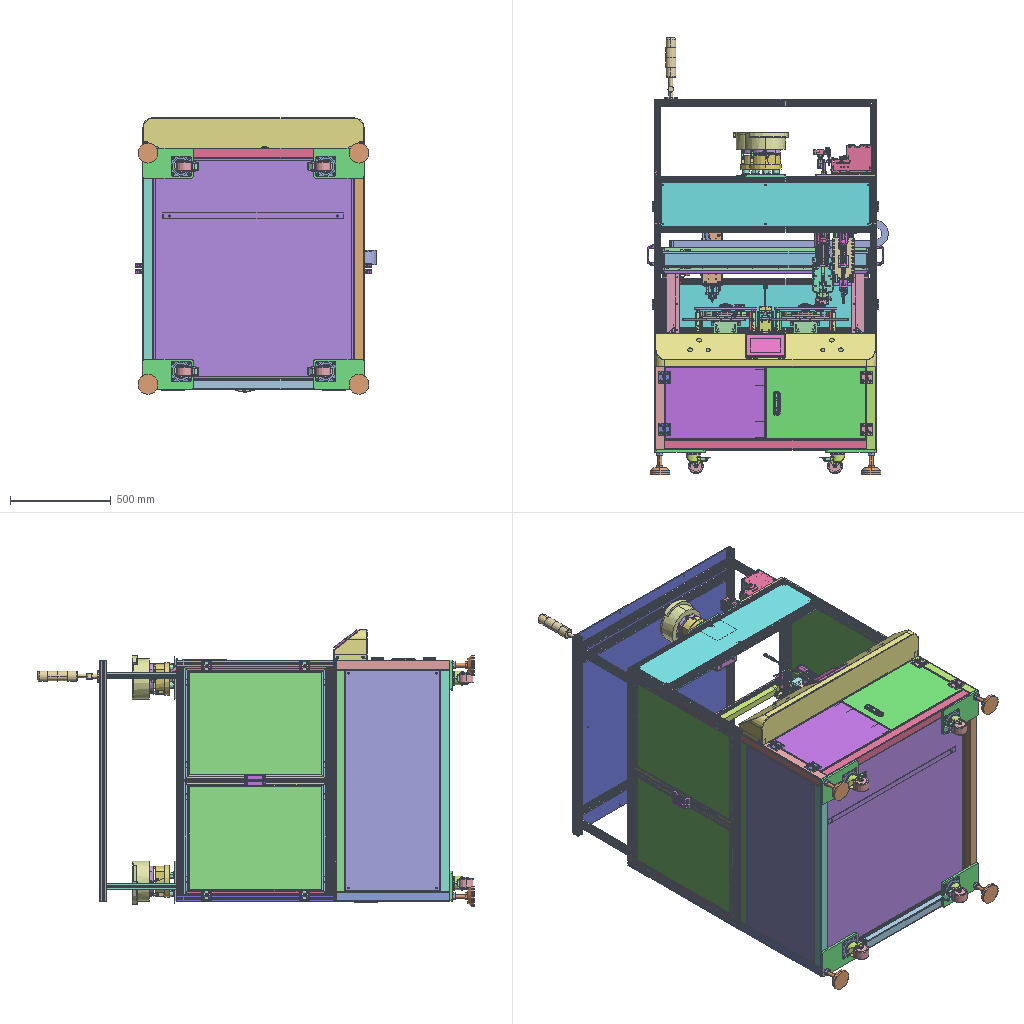Assembly | SolidWorks | 335 different items | 808 placed | box 1197 x 2172 x 1376 mm
Parts list (item | name | quantity | parent item | size | volume | features):
1 | 2MANIFOLD_SOLID_BREP_106 | x1 | - | - | - | -
2 | 2MANIFOLD_SOLID_BREP_107 | x1 | - | - | - | -
3 | 48-0003-001 Fuma Feeder | x1 | - | - | - | -
4 | (subassembly) | x2 | - | - | 2926027 mm3 | features InContextFeatHolder 1, LocalLPattern 1
5 | (subassembly) | x1 | in 48 | 106 x 347.75 x 115.5 mm | 813815 mm3 | -
6 | (subassembly) | x1 | in 48 | 118 x 296 x 169.5 mm | 901721 mm3 | features CompositeCurve 3
7 | (subassembly) | x1 | in 48 | - | 1242766 mm3 | features LocalLPattern 2, ReferencePattern 2, CompositeCurve 1
8 | (subassembly) | x1 | in 48 | - | 1493207 mm3 | features InContextFeatHolder 2, LocalLPattern 1, ReferencePattern 1
9 | (subassembly) | x2 | in 39 | 204.5 x 53 x 57 mm | 221430 mm3 | features CompositeCurve 1
10 | (subassembly) | x1 | in 5 | 163 x 64 x 71 mm | 272999 mm3 | features CompositeCurve 1
11 | (subassembly) | x1 | in 8 | 177 x 64 x 71 mm | 281305 mm3 | -
12 | (subassembly) | x4 | in 48 | 34 x 24 x 801 mm | 156547 mm3 | -
13 | (subassembly) | x1 | - | 160 x 158.001 x 310 mm | 1338981 mm3 | -
14 | (subassembly) | x1 | in 13 | - | - | -
15 | (subassembly) | x1 | in 5 | 75.5 x 39 x 43.25 mm | 30245 mm3 | -
16 | (subassembly) | x1 | in 13 | - | - | -
17 | (subassembly) | x1 | in 13 | - | - | -
18 | (subassembly) | x2 | in 39 | 72 x 24 x 16.5 mm | 14994 mm3 | features CompositeCurve 1
19 | (subassembly) | x2 | in 7 | 27 x 13 x 214 mm | 32172 mm3 | -
20 | (subassembly) | x2 | in 47, 52 | 128 x 25.22 x 23.366 mm | 18624 mm3 | features CompositeCurve 2
21 | (subassembly) | x1 | in 25 | 334 x 47.242 x 35.2 mm | 41085 mm3 | -
22 | (subassembly) | x2 | in 13 | 82 x 58 x 26 mm | 65223 mm3 | -
23 | (subassembly) | x2 | in 33 | 215 x 212 x 215 mm | 2165561 mm3 | -
24 | (subassembly) | x4 | in 28 | 109 x 58 x 20 mm | 97636 mm3 | -
25 | (subassembly) | x1 | in 48 | 108.9 x 604.66 x 99 mm | 644480 mm3 | -
26 | (subassembly) | x1 | in 49 | 532 x 358 x 55 mm | 405860 mm3 | -
27 | (subassembly) | x1 | in 49 | 549 x 358 x 41 mm | 436245 mm3 | -
28 | (subassembly) | x2 | in 4 | - | 4562071 mm3 | features InContextFeatHolder 23, LocalLPattern 2, ReferencePattern 2
29 | (subassembly) | x1 | in 49 | 1150 x 697 x 1255 mm | 10713372 mm3 | features ReferencePattern 18, MirrorCompFeat 5
30 | (subassembly) | x4 | in 38 | 51 x 717 x 593 mm | 2782623 mm3 | -
31 | (subassembly) | x1 | in 7 | 57.15 x 69.65 x 99 mm | 128417 mm3 | -
32 | (subassembly) | x5 | in 4, 6, 48 | 57.15 x 69.65 x 131 mm | 178571 mm3 | -
33 | (subassembly) | x2 | - | 215 x 224 x 215 mm | 2633576 mm3 | features ReferencePattern 12, MirrorCompFeat 2
34 | (subassembly) | x1 | in 25 | 28.124 x 80.028 x 32.009 mm | 13678 mm3 | features MirrorCompFeat 1, ReferencePattern 1
35 | (subassembly) | x1 | in 7 | 15 x 15 x 281 mm | 43646 mm3 | -
36 | (subassembly) | x2 | in 47, 52 | 27 x 13 x 80 mm | 13505 mm3 | -
37 | (subassembly) | x1 | in 5 | 24 x 50 x 40 mm | 9876 mm3 | -
38 | (subassembly) | x1 | - | - | 31701876 mm3 | features ReferencePattern 32, MirrorCompFeat 9, InContextFeatHolder 2, LocalLPattern 1
39 | (subassembly) | x2 | in 8, 48 | 174 x 106 x 364.833 mm | 559956 mm3 | features InContextFeatHolder 16
40 | (subassembly) | x2 | in 8 | 27 x 13 x 140 mm | 25516 mm3 | features LocalLPattern 1, ReferencePattern 1
41 | (subassembly) | x4 | in 28 | 50.06 x 40.7 x 50.06 mm | 29200 mm3 | -
42 | (subassembly) | x2 | in 28 | 63.5 x 60 x 65 mm | 47283 mm3 | features InContextFeatHolder 3
43 | (subassembly) | x2 | in 39 | - | - | -
44 | (subassembly) | x4 | in 28 | 50.005 x 46.2 x 50.005 mm | 37880 mm3 | features InContextFeatHolder 3
45 | (subassembly) | x2 | in 13 | - | - | -
46 | (subassembly) | x2 | in 13 | - | - | -
47 | (subassembly) | x1 | - | 247.423 x 78.5 x 242 mm | 390911 mm3 | features InContextFeatHolder 6, CompositeCurve 2
48 | (subassembly) | x1 | - | - | - | features InContextFeatHolder 20, ReferencePattern 6, LocalLPattern 2, AEMSimFeature 1, MirrorCompFeat 1
49 | (subassembly) | x1 | - | - | 25832975 mm3 | features InContextFeatHolder 16, ReferencePattern 13, MirrorCompFeat 5
50 | (subassembly) | x1 | - | - | - | -
51 | (subassembly) | x5 | in 4, 6, 48 | 86 x 30 x 36 mm | 32834 mm3 | -
52 | (subassembly) | x1 | - | 247.56 x 78.5 x 242 mm | 391168 mm3 | features CompositeCurve 2
53 | (subassembly) | x4 | in 13 | - | - | -
54 | (subassembly) | x8 | in 30 | 50 x 50 x 12 mm | 15792 mm3 | -
55 | - | x1 | in 6 | 15 x 15 x 180 mm | 39722 mm3 | features ICE 2, Extrusion 1, LPattern 1
56 | - | x2 | in 48 | 83 x 297.5 x 153 mm | 132510 mm3 | features ICE 3, Fillet 2, Shell 2, Chamfer 1, Extrusion 1, HoleWzd 1
57 | - | x4 | in 4 | 122 x 65.5 x 4 mm | 31619 mm3 | features Extrusion 1, Fillet 1
58 | - | x4 | in 4, 48 | 14 x 33 x 12 mm | 507.507 mm3 | features MoveFace 7, ICE 2, BaseBody 1, Fillet 1
59 | - | x4 | in 4, 48 | 19 x 20 x 50 mm | 3170 mm3 | features Fillet 3, ICE 2, ExtruThin 1
60 | - | x4 | in 38 | 3 x 60 x 50 mm | 5947 mm3 | features HoleWzd 2, Fillet 1, FlatPattern 1, ICE 1, SMBaseFlange 1, SheetMetal 1
61 | - | x1 | in 6 | 30 x 50 x 100 mm | 12860 mm3 | features HoleWzd 2, EdgeFlange 1, Fillet 1, FlatPattern 1, SMBaseFlange 1, SheetMetal 1
62 | - | x2 | in 47, 52 | 5 x 12 x 25 mm | 1176 mm3 | features Fillet 4, ICE 4, Cut 1, Extrusion 1, HoleWzd 1
63 | - | x4 | in 47, 52 | 3 x 67 x 43.5 mm | 6128 mm3 | features ICE 5, Fillet 4, Extrusion 1, HoleWzd 1, LPattern 1
64 | - | x2 | in 47, 52 | 3 x 42 x 25 mm | 2502 mm3 | features Fillet 3, ICE 3, Cut 1, Extrusion 1, HoleWzd 1
65 | - | x2 | in 47, 52 | 1 x 48 x 65 mm | 2915 mm3 | features ICE 8, Fillet 2, Chamfer 1, Extrusion 1, HoleWzd 1
66 | - | x1 | in 25 | 34 x 19.5 x 56.8 mm | 30598 mm3 | features ICE 2, Extrusion 1
67 | - | x2 | in 33 | 184 x 160 x 140 mm | 320249 mm3 | features Fillet 2, Extrusion 1, ICE 1
68 | - | x4 | in 39 | 3 x 36 x 65 mm | 4945 mm3 | features Fillet 2, HoleWzd 2, ICE 2, Extrusion 1
69 | - | x2 | in 39 | 33 x 59 x 3 mm | 3614 mm3 | features Cut 4, ICE 4, Fillet 3, MoveFace 2, Extrusion 1, HoleWzd 1
70 | - | x2 | in 39 | 35 x 23 x 3 mm | 2147 mm3 | features Fillet 2, MoveFace 2, Extrusion 1, ICE 1
71 | - | x2 | in 39 | 14.5 x 3 x 15 mm | 477.667 mm3 | features Extrusion 1, Fillet 1, ICE 1
72 | - | x2 | in 39 | 43 x 37 x 0.8 mm | 1152 mm3 | features ICE 5, HoleWzd 2, Cut 1, Extrusion 1, Fillet 1, MirrorPattern 1, MoveFace 1
73 | - | x1 | in 7 | 30 x 50 x 66 mm | 9795 mm3 | features HoleWzd 2, EdgeFlange 1, Fillet 1, FlatPattern 1, SMBaseFlange 1, SheetMetal 1
74 | - | x1 | in 7 | 33.8 x 20 x 11 mm | 767.773 mm3 | features EdgeFlange 2, ICE 2, Fillet 1, FlatPattern 1, SMBaseFlange 1, SheetMetal 1
75 | - | x1 | in 25 | 25 x 53 x 20 mm | 8091 mm3 | features ICE 7, HoleWzd 4, 3DProfileFeature 2, Chamfer 2, Extrusion 1, Fillet 1, RevCut 1, Revolution 1
76 | - | x2 | in 5 | 12 x 120 x 12 mm | 13432 mm3 | features Chamfer 1, Extrusion 1, HoleWzd 1, ICE 1
77 | - | x2 | in 39 | 5.7 x 10.3 x 5.7 mm | 17.455 mm3 | features Helix 1, ICE 1, Sweep 1
78 | - | x1 | in 5 | 24 x 65 x 25 mm | 25326 mm3 | features HoleWzd 3, ICE 2, Chamfer 1, Extrusion 1, MirrorPattern 1
79 | - | x1 | in 37 | 11 x 32 x 11 mm | 1736 mm3 | features Chamfer 5, ICE 4, HoleWzd 3, RevCut 2, Extrusion 1
80 | - | x2 | in 39 | 10 x 60 x 10 mm | 1412 mm3 | features Chamfer 1, Extrusion 1, Fillet 1, ICE 1
81 | - | x2 | in 39 | 3 x 145 x 3 mm | 797.28 mm3 | features ICE 4, Chamfer 2, MoveFace 2, Extrusion 1
82 | - | x2 | in 39 | 15 x 13 x 30 mm | 3613 mm3 | features ICE 4, Chamfer 1, Extrusion 1, HoleWzd 1
83 | - | x2 | in 48 | 150 x 300 x 20 mm | 887361 mm3 | features HoleWzd 5, MirrorPattern 2, Chamfer 1, Extrusion 1
84 | - | x1 | in 48 | 15 x 150 x 1018 mm | 2102309 mm3 | features HoleWzd 6, ICE 3, MirrorPattern 2, Chamfer 1, Extrusion 1, Fillet 1
85 | - | x1 | in 48 | 1000 x 118 x 12 mm | 1222730 mm3 | features HoleWzd 11, ICE 3, MirrorPattern 3, Chamfer 2, Cut 2, Fillet 2, LPattern 2, MoveFace 2, Extrusion 1
86 | - | x4 | in 48 | 75 x 4 x 8 mm | 2157 mm3 | features Chamfer 5, ICE 4, HoleWzd 2, Extrusion 1, Fillet 1
87 | - | x1 | in 48 | 150 x 133 x 15 mm | 253404 mm3 | features HoleWzd 4, ICE 3, Extrusion 1, Fillet 1, MirrorPattern 1
88 | - | x2 | in 39 | 13.6 x 2 x 2 mm | 42.623 mm3 | features Extrusion 1, Fillet 1
89 | - | x2 | in 48 | 65 x 35 x 85 mm | 63871 mm3 | features HoleWzd 5, ICE 3, Extrusion 1
90 | - | x2 | in 48 | 70 x 112 x 15 mm | 96794 mm3 | features HoleWzd 8, ICE 4, MirrorPattern 2, Extrusion 1
91 | - | x4 | in 48 | 12 x 70 x 45 mm | 30841 mm3 | features HoleWzd 5, Extrusion 1, MirrorPattern 1
92 | - | x2 | in 48 | 50 x 95 x 20 mm | 89595 mm3 | features HoleWzd 2, Chamfer 1, Extrusion 1
93 | - | x1 | in 48 | 150 x 133 x 15 mm | 252829 mm3 | features HoleWzd 4, ICE 3, Extrusion 1, Fillet 1, MirrorPattern 1
94 | - | x4 | in 4, 48 | 50 x 16 x 5.5 mm | 4295 mm3 | features Chamfer 1, Extrusion 1, HoleWzd 1
95 | - | x2 | in 4 | 150 x 200 x 10 mm | 295428 mm3 | features HoleWzd 3, ICE 3, Extrusion 1, Fillet 1, LPattern 1
96 | - | x1 | in 5 | 106 x 235 x 10 mm | 238418 mm3 | features HoleWzd 7, ICE 5, Fillet 2, Extrusion 1, LPattern 1, MirrorPattern 1, MoveFace 1
97 | - | x1 | in 5 | 82 x 10 x 82 mm | 53941 mm3 | features HoleWzd 7, Extrusion 1, Fillet 1, ICE 1, MirrorPattern 1
98 | - | x1 | in 5 | 26 x 35 x 15.8 mm | 2299 mm3 | features ICE 10, Fillet 6, Chamfer 1, Extrusion 1, HoleWzd 1, MoveFace 1
99 | - | x2 | in 48 | 30 x 24 x 30 mm | 11200 mm3 | features ICE 11, Chamfer 4, CirPattern 1, HoleWzd 1, Revolution 1
100 | - | x1 | in 5 | 26 x 35 x 15.8 mm | 2299 mm3 | features MirrorStock 1
101 | - | x1 | in 5 | 65 x 10 x 32 mm | 16925 mm3 | features HoleWzd 3, ICE 3, Extrusion 1, Fillet 1
102 | - | x1 | in 5 | 95 x 12 x 100 mm | 64491 mm3 | features HoleWzd 6, ICE 3, Fillet 2, Extrusion 1
103 | - | x1 | in 8 | 72 x 10 x 64 mm | 33293 mm3 | features HoleWzd 5, ICE 5, Fillet 2, Extrusion 1
104 | - | x1 | in 37 | 24 x 24 x 40 mm | 8141 mm3 | features ICE 7, Chamfer 4, HoleWzd 4, Extrusion 1, RevCut 1
105 | - | x1 | in 8 | 95 x 170.5 x 10 mm | 143560 mm3 | features HoleWzd 8, ICE 8, Fillet 4, MoveFace 2, Cut 1, Extrusion 1, MirrorPattern 1
106 | - | x1 | in 8 | 180 x 190 x 10 mm | 333166 mm3 | features HoleWzd 6, ICE 2, Extrusion 1, Fillet 1, LPattern 1
107 | - | x3 | in 4, 6 | 86 x 58 x 5 mm | 19221 mm3 | features ICE 5, HoleWzd 4, 3DProfileFeature 2, MirrorPattern 2, Chamfer 1, Cut 1, Extrusion 1, LPattern 1
108 | - | x1 | in 6 | 238.67 x 16.67 x 12 mm | 3738 mm3 | features Extrusion 1
109 | - | x1 | in 6 | 86 x 24 x 36 mm | 22794 mm3 | features ICE 7, Chamfer 1, Extrusion 1, RevCut 1
110 | - | x2 | in 6 | 100 x 65 x 8 mm | 46552 mm3 | features Chamfer 4, MoveFace 3, Fillet 2, HoleWzd 2, ICE 2, Extrusion 1
111 | - | x2 | in 47, 52 | 12 x 55 x 140 mm | 81002 mm3 | features ICE 2, Chamfer 1, Extrusion 1, HoleWzd 1, MirrorPattern 1
112 | - | x4 | in 47, 52 | 55 x 60 x 10 mm | 32595 mm3 | features Extrusion 1, HoleWzd 1, MirrorPattern 1
113 | - | x2 | in 47, 52 | 12 x 55 x 152 mm | 91517 mm3 | features HoleWzd 6, ICE 5, MirrorPattern 2, Chamfer 1, Cut 1, Extrusion 1
114 | - | x6 | in 39, 47, 52 | 20 x 10 x 8 mm | 1332 mm3 | features HoleWzd 2, Extrusion 1, ICE 1, MoveFace 1
115 | - | x2 | in 47, 52 | 10 x 55 x 35 mm | 16084 mm3 | features HoleWzd 3, Chamfer 1, Extrusion 1, ICE 1, MirrorPattern 1
116 | - | x2 | in 47, 52 | 10 x 48 x 20 mm | 8641 mm3 | features Extrusion 1, HoleWzd 1
117 | - | x3 | in 39, 47 | 25 x 55 x 12 mm | 15520 mm3 | features ICE 4, Chamfer 2, Fillet 2, HoleWzd 2, MirrorPattern 2, Extrusion 1
118 | - | x1 | in 47 | 20 x 48 x 65 mm | 52206 mm3 | features ICE 6, HoleWzd 3, Chamfer 2, Fillet 2, Extrusion 1, MoveFace 1
119 | - | x1 | in 52 | 20 x 48 x 65 mm | 52425 mm3 | features ICE 6, HoleWzd 3, Chamfer 2, Fillet 2, Extrusion 1, MoveFace 1
120 | - | x3 | in 39, 52 | 25 x 55 x 12 mm | 15456 mm3 | features ICE 4, Chamfer 2, Fillet 2, HoleWzd 2, MirrorPattern 2, Extrusion 1
121 | - | x1 | in 8 | 96 x 120 x 10 mm | 109019 mm3 | features HoleWzd 2, Extrusion 1, Fillet 1, ICE 1
122 | - | x2 | in 39 | 7 x 7 x 42.5 mm | 1702 mm3 | features Chamfer 3, ICE 3, Extrusion 1, MoveFace 1
123 | - | x2 | in 39 | 52 x 37 x 19 mm | 25597 mm3 | features HoleWzd 8, ICE 8, MoveFace 8, Chamfer 2, Extrusion 1, Fillet 1, MirrorPattern 1, RefAxis 1
124 | - | x2 | in 39 | 7 x 8.44 x 8 mm | 333.679 mm3 | features ICE 5, Chamfer 2, Extrusion 1, MoveFace 1
125 | - | x2 | in 39 | 5 x 8.4 x 7.9 mm | 224.151 mm3 | features ICE 5, Chamfer 2, MoveFace 2, Extrusion 1
126 | - | x2 | in 39 | 22 x 12.5 x 10 mm | 1861 mm3 | features HoleWzd 2, ICE 2, Chamfer 1, Extrusion 1, MoveFace 1
127 | - | x2 | in 39 | 43 x 37 x 12 mm | 14568 mm3 | features HoleWzd 6, ICE 4, MoveFace 2, Chamfer 1, Extrusion 1, LPattern 1, RefAxis 1
128 | - | x2 | in 39 | 33 x 15 x 45 mm | 11629 mm3 | features Chamfer 1, Extrusion 1, HoleWzd 1, ICE 1
129 | - | x2 | in 39 | 95 x 12 x 63 mm | 36710 mm3 | features HoleWzd 7, ICE 3, Fillet 2, Extrusion 1
130 | - | x2 | in 39 | 106 x 235 x 10 mm | 201663 mm3 | features ICE 18, HoleWzd 12, Fillet 5, MoveFace 3, LPattern 2, MirrorPattern 2, Extrusion 1
131 | - | x2 | in 39 | 96 x 211.5 x 10 mm | 163638 mm3 | features ICE 21, HoleWzd 16, Fillet 5, MoveFace 3, LPattern 2, MirrorPattern 2, Chamfer 1, Extrusion 1
132 | - | x1 | in 7 | 100 x 75 x 8 mm | 49957 mm3 | features Cut 2, HoleWzd 2, Chamfer 1, Extrusion 1, Fillet 1, ICE 1
133 | - | x1 | in 7 | 100 x 71.5 x 8 mm | 49163 mm3 | features Chamfer 1, Cut 1, Extrusion 1, Fillet 1, HoleWzd 1, ICE 1
134 | - | x1 | in 7 | 86 x 61.5 x 12 mm | 38021 mm3 | features HoleWzd 5, ICE 5, Chamfer 4, MoveFace 3, Extrusion 1
135 | - | x1 | in 7 | 86 x 61.5 x 15 mm | 44493 mm3 | features ICE 7, HoleWzd 4, Chamfer 3, MoveFace 2, Extrusion 1
136 | - | x1 | in 7 | 106 x 56 x 80 mm | 252675 mm3 | features ICE 9, HoleWzd 7, Chamfer 4, CirPattern 2, Cut 2, Extrusion 1, LPattern 1
137 | - | x3 | in 38 | 215 x 1038 x 6 mm | 1337506 mm3 | features Extrusion 1, Fillet 1, HoleWzd 1
138 | - | x1 | in 38 | 1100 x 6 x 1200 mm | 7913109 mm3 | features HoleWzd 2, ICE 2, Extrusion 1, Fillet 1
139 | - | x4 | in 30 | 6 x 677 x 528 mm | 2144688 mm3 | features Chamfer 1, Extrusion 1
140 | - | x2 | in 33 | 200 x 12 x 200 mm | 468015 mm3 | features Cut 1, Extrusion 1, Fillet 1
141 | - | x1 | in 6 | 45 x 8 x 15 mm | 5130 mm3 | features Extrusion 1, HoleWzd 1, ICE 1
142 | - | x2 | in 7 | 12 x 12 x 15 mm | 1371 mm3 | features Extrusion 1, HoleWzd 1
143 | - | x2 | in 48 | 79 x 6 x 1020 mm | 209920 mm3 | features Cut 1, Extrusion 1, MirrorPattern 1
144 | - | x2 | in 4 | 143.4 x 35.1 x 60 mm | 99066 mm3 | features HoleWzd 8, MirrorPattern 5, ICE 3, Chamfer 1, Extrusion 1, LPattern 1
145 | - | x2 | in 4 | 120 x 12 x 1000 mm | 423626 mm3 | features Extrusion 1, HoleWzd 1, ICE 1, MirrorPattern 1
146 | - | x1 | in 38 | 1100 x 780 x 1200 mm | 5922757 mm3 | features ICE 14, 3DProfileFeature 2, HoleWzd 2, WeldMemberFeat 2, WeldmentFeature 1
147 | - | x4 | in 30 | 30 x 15 x 717 mm | 163021 mm3 | features Extrusion 1, HoleWzd 1, ICE 1
148 | - | x4 | in 30 | 30 x 15 x 717 mm | 163444 mm3 | features Extrusion 1, HoleWzd 1, ICE 1
149 | - | x4 | in 29 | 100 x 106 x 139 mm | 279325 mm3 | features BaseBody 5
150 | - | x8 | in 30 | 30 x 15 x 568 mm | 128082 mm3 | features Extrusion 1, HoleWzd 1, ICE 1
151 | - | x4 | in 38 | 1040 x 30 x 30 mm | 414964 mm3 | features WeldMemberFeat 1, WeldmentFeature 1
152 | - | x1 | in 6 | 100 x 46 x 280 mm | 353239 mm3 | features HoleWzd 7, ICE 5, MirrorPattern 5, 3DProfileFeature 3, Fillet 3, LPattern 3, Cut 2, Chamfer 1, Extrusion 1
153 | - | x1 | in 6 | 106 x 38 x 60 mm | 90816 mm3 | features HoleWzd 7, 3DProfileFeature 4, ICE 4, Chamfer 1, Extrusion 1, LPattern 1, MirrorPattern 1, MoveFace 1
154 | - | x1 | in 6 | 79 x 6 x 296 mm | 60805 mm3 | features Cut 1, Extrusion 1, MirrorPattern 1
155 | - | x1 | in 7 | 100 x 46 x 306 mm | 422449 mm3 | features HoleWzd 8, ICE 3, 3DProfileFeature 1, Extrusion 1, LPattern 1, MirrorPattern 1
156 | - | x1 | in 7 | 79 x 6 x 306 mm | 62238 mm3 | features ICE 4, Extrusion 1, HoleWzd 1
157 | - | x1 | in 7 | 6 x 9 x 200 mm | 5872 mm3 | features ICE 3, Extrusion 1
158 | - | x5 | in 51 | 86 x 24 x 36 mm | 22794 mm3 | features ICE 7, Chamfer 1, Extrusion 1, RevCut 1
159 | - | x2 | in 4 | 30 x 24 x 30 mm | 11209 mm3 | features ICE 12, Chamfer 4, CirPattern 1, HoleWzd 1, Revolution 1
160 | - | x1 | in 48 | 781.5 x 119 x 54 mm | 397201 mm3 | features ICE 12, Fillet 2, HoleWzd 2, Shell 1, Sweep 1
161 | - | x5 | in 51 | 30 x 21 x 30 mm | 8531 mm3 | features Chamfer 2, ICE 2, MirrorPattern 1, Revolution 1
162 | - | x4 | in 4 | 45 x 8 x 15 mm | 5130 mm3 | features Extrusion 1, HoleWzd 1, ICE 1
163 | - | x2 | in 4 | 100 x 46 x 1000 mm | 1360190 mm3 | features HoleWzd 6, ICE 6, MirrorPattern 4, Fillet 3, LPattern 3, Chamfer 1, Extrusion 1
164 | - | x2 | in 28 | 15 x 215 x 215 mm | 479091 mm3 | features ICE 5, HoleWzd 3, Cut 2, Fillet 2, LPattern 2, Chamfer 1, Extrusion 1, RefAxis 1, RevCut 1
165 | - | x2 | in 28 | 10.7 x 214.9 x 214.8 mm | 326451 mm3 | features MoveCopyBody 6, ICE 5, Fillet 2, LPattern 2, MoveFace 2, Chamfer 1, Cut 1, Extrusion 1, Stock 1
166 | - | x2 | in 28 | 10.7 x 214.9 x 214.8 mm | 309606 mm3 | features ICE 6, MoveCopyBody 6, Cut 3, Fillet 3, Chamfer 1, Extrusion 1, LPattern 1, MoveFace 1, Stock 1
167 | - | x2 | in 28 | 13.1 x 214.9 x 214.8 mm | 329886 mm3 | features ICE 7, MoveCopyBody 6, Fillet 3, Cut 2, Chamfer 1, Extrusion 1, LPattern 1, MoveFace 1, Stock 1
168 | - | x2 | in 28 | 10 x 225 x 237 mm | 510039 mm3 | features HoleWzd 6, Chamfer 2, MirrorPattern 2, MoveFace 2, Extrusion 1, ICE 1
169 | - | x2 | in 28 | 25 x 225 x 10 mm | 52898 mm3 | features Chamfer 2, HoleWzd 2, Extrusion 1, Fillet 1
170 | - | x2 | in 28 | 25 x 10 x 210 mm | 50226 mm3 | features Extrusion 1, HoleWzd 1, ICE 1
171 | - | x2 | in 28 | 8 x 215 x 311 mm | 385506 mm3 | features Cut 2, Fillet 2, ICE 2, MirrorPattern 2, MoveFace 2, Chamfer 1, Extrusion 1, LPattern 1
172 | - | x4 | in 28 | 98 x 10 x 157.5 mm | 116638 mm3 | features HoleWzd 4, Chamfer 1, Extrusion 1, Fillet 1, ICE 1
173 | - | x2 | in 28 | 25 x 225 x 10 mm | 52898 mm3 | features MirrorStock 1
174 | - | x3 | in 28 | 10 x 35 x 120 mm | 41153 mm3 | features Chamfer 1, Extrusion 1, HoleWzd 1, ICE 1, LPattern 1
175 | - | x2 | in 28 | 25 x 215 x 215 mm | 792326 mm3 | features ICE 12, MoveCopyBody 7, LPattern 6, MoveFace 5, Chamfer 4, Cut 2, Fillet 2, Stock 2, Extrusion 1, HoleWzd 1
176 | - | x2 | in 28 | 98 x 10 x 157.5 mm | 116638 mm3 | features MirrorStock 1
177 | - | x2 | in 28 | 25 x 215 x 215 mm | 773722 mm3 | features ICE 14, MoveCopyBody 7, LPattern 5, MoveFace 5, Chamfer 3, Cut 2, Stock 2, Extrusion 1, HoleWzd 1
178 | - | x2 | in 28 | 25 x 215 x 215 mm | 796831 mm3 | features ICE 14, MoveCopyBody 7, MoveFace 6, Chamfer 4, LPattern 4, Cut 3, Fillet 3, Stock 2, Extrusion 1, HoleWzd 1
179 | - | x1 | in 6 | 19 x 17 x 50 mm | 3062 mm3 | features Fillet 3, ICE 2, ExtruThin 1
180 | - | x1 | in 6 | 50 x 16 x 3 mm | 2365 mm3 | features Chamfer 1, Extrusion 1, HoleWzd 1
181 | - | x4 | in 44 | 16.9 x 32 x 32 mm | 11867 mm3 | features ICE 6, Cut 1, Extrusion 1, Fillet 1
182 | - | x1 | in 6 | 14 x 25 x 12 mm | 411.507 mm3 | features MoveFace 3, ICE 2, BaseBody 1, Fillet 1
183 | - | x1 | in 6 | 30 x 24 x 30 mm | 11209 mm3 | features ICE 12, Chamfer 4, CirPattern 1, HoleWzd 1, Revolution 1
184 | - | x2 | in 25 | 20 x 16 x 16 mm | 3358 mm3 | features Extrusion 1
185 | - | x1 | in 25 | 40 x 17 x 58.5 mm | 18418 mm3 | features ICE 9, Chamfer 6, HoleWzd 5, MirrorPattern 3, Fillet 2, MoveFace 2, Extrusion 1
186 | - | x2 | in 48 | 880.84 x 28.34 x 15 mm | 31689 mm3 | features Extrusion 1
187 | - | x1 | in 35 | 15 x 15 x 281 mm | 43646 mm3 | features RevCut 4, Chamfer 2, Extrusion 1, ICE 1
188 | - | x1 | - | 18 x 55 x 99.9 mm | 49289 mm3 | features BaseBody 1
189 | - | x2 | in 6, 7 | 8.882 x 97 x 8 mm | 1277 mm3 | features BaseBody 3, ICE 1, RefAxis 1
190 | - | x1 | in 10 | 8 x 31.177 x 27 mm | 3647 mm3 | features BaseBody 1
191 | - | x1 | in 11 | 8 x 31.177 x 27 mm | 3647 mm3 | features BaseBody 1
192 | - | x6 | in 41, 42 | 14.5 x 33 x 33 mm | 10024 mm3 | features Cut 2, ICE 2, CirPattern 1, Extrusion 1
193 | - | x1 | in 10 | 11 x 31.177 x 27 mm | 4519 mm3 | features BaseBody 1
194 | - | x1 | in 10 | 31 x 36 x 36 mm | 21772 mm3 | features BaseBody 1
195 | - | x1 | in 11 | 41 x 36 x 36 mm | 28650 mm3 | features BaseBody 1
196 | - | x1 | in 11 | 177 x 50 x 50 mm | 73758 mm3 | features BaseBody 1
197 | - | x1 | in 11 | 80.5 x 71 x 64 mm | 175247 mm3 | features BaseBody 1
198 | - | x1 | in 10 | 163 x 50 x 50 mm | 86233 mm3 | features BaseBody 1
199 | - | x1 | in 10 | 70.5 x 71 x 64 mm | 156826 mm3 | features BaseBody 1
200 | - | x2 | in 20 | 107 x 18 x 18 mm | 12758 mm3 | features BaseBody 1
201 | - | x2 | in 20 | 110.9 x 11.5 x 11.5 mm | 4064 mm3 | features BaseBody 1
202 | - | x1 | in 13 | - | - | features RefSurface 77
203 | - | x2 | in 20 | 6 x 25.403 x 22 mm | 1471 mm3 | features BaseBody 1
204 | - | x2 | in 20 | 5 x 11.547 x 10 mm | 331.011 mm3 | features BaseBody 1
205 | - | x1 | in 21 | 6 x 25.403 x 22 mm | 1471 mm3 | features BaseBody 1
206 | - | x1 | in 21 | 5 x 11.547 x 10 mm | 331.011 mm3 | features BaseBody 1
207 | - | x1 | in 21 | 334 x 15.5 x 15.5 mm | 11530 mm3 | features BaseBody 1
208 | - | x1 | in 21 | 167 x 20 x 20 mm | 22187 mm3 | features BaseBody 1
209 | - | x1 | in 21 | 5 x 11.547 x 10 mm | 331.011 mm3 | features BaseBody 1
210 | - | x1 | in 21 | 66 x 15 x 15 mm | 8114 mm3 | features BaseBody 1
211 | - | x2 | in 22 | 49 x 26 x 58 mm | 50658 mm3 | features BaseBody 1
212 | - | x2 | in 22 | 59.5 x 22 x 56 mm | 14565 mm3 | features BaseBody 1
213 | - | x1 | in 38 | 900 x 35 x 34 mm | 955428 mm3 | features Extrusion 1, HoleWzd 1, ICE 1, MirrorPattern 1
214 | - | x4 | in 24 | 99 x 20 x 58 mm | 74621 mm3 | features BaseBody 1
215 | - | x4 | in 24 | 103.6 x 18 x 56 mm | 23014 mm3 | features BaseBody 1
216 | - | x2 | in 39 | 6 x 6 x 55 mm | 1555 mm3 | features Extrusion 1
217 | - | x4 | in 44 | 32 x 33.3 x 32 mm | 14832 mm3 | features ICE 2, BaseBody 1, MoveFace 1
218 | - | x6 | in 41, 42 | 33 x 35.1 x 33 mm | 19096 mm3 | features MoveFace 3, BaseBody 1, CirPattern 1, HoleWzd 1
219 | - | x1 | in 8 | 17 x 19.6 x 45 mm | 6216 mm3 | features BaseBody 1, MoveFace 1
220 | - | x2 | in 47, 52 | 15.5 x 15.5 x 18 mm | 2342 mm3 | features BaseBody 1
221 | - | x1 | in 13 | 98 x 66 x 12 mm | 42190 mm3 | features ICE 6, HoleWzd 4, Chamfer 2, Extrusion 1, MirrorPattern 1
222 | - | x4 | in 41 | 1.99 x 13.6 x 1.99 mm | 41.809 mm3 | features BaseBody 1
223 | - | x2 | in 28 | 12 x 31.537 x 120 mm | 3389 mm3 | features Fillet 4, Extrusion 1, ICE 1
224 | - | x4 | in 13 | 13 x 6 x 13 mm | 944.273 mm3 | features Chamfer 1, Extrusion 1, HoleWzd 1
225 | - | x1 | in 13 | 30 x 12 x 62 mm | 15056 mm3 | features ICE 3, HoleWzd 2, Chamfer 1, Extrusion 1, MirrorPattern 1
226 | - | x1 | in 13 | 126 x 12 x 25 mm | 32289 mm3 | features ICE 4, Chamfer 1, Extrusion 1, HoleWzd 1, MirrorPattern 1
227 | - | x1 | in 5 | 53 x 53 x 22 mm | 15531 mm3 | features ICE 3, Chamfer 1, Extrusion 1
228 | - | x1 | in 5 | 15 x 15 x 47 mm | 1444 mm3 | features 3DProfileFeature 1, Helix 1, RefAxis 1, Sweep 1
229 | - | x8 | in 48 | 53 x 53 x 52 mm | 37709 mm3 | features ICE 3, Chamfer 1, Extrusion 1
230 | - | x1 | in 38 | 60 x 307 x 60 mm | 453785 mm3 | features BaseBody 1
231 | - | x1 | in 13 | 160 x 12 x 300 mm | 482018 mm3 | features HoleWzd 12, ICE 6, Chamfer 1, Extrusion 1, Fillet 1, MirrorPattern 1
232 | - | x1 | in 13 | 14 x 25 x 15 mm | 2174 mm3 | features ICE 6, Chamfer 2, RevCut 2, Extrusion 1, MirrorPattern 1
233 | - | x4 | in 41 | 1.99 x 13.6 x 1.99 mm | 41.809 mm3 | features BaseBody 1
234 | - | x1 | in 13 | 14 x 29 x 15 mm | 2672 mm3 | features Chamfer 4, ICE 4, Extrusion 1, HoleWzd 1
235 | - | x1 | in 13 | 42 x 10 x 29 mm | 6453 mm3 | features HoleWzd 3, ICE 3, Fillet 2, Chamfer 1, Extrusion 1
236 | - | x1 | in 13 | 56 x 25 x 26 mm | 11259 mm3 | features ICE 5, Fillet 2, HoleWzd 2, Chamfer 1, Extrusion 1
237 | - | x1 | in 49 | 200 x 145 x 43 mm | 1064774 mm3 | features ICE 5, Fillet 3, Extrusion 1
238 | - | x1 | in 25 | - | - | features BaseBody 5, Fillet 2, ICE 1, RefSurface 1
239 | - | x1 | in 5 | 118 x 5 x 5 mm | 2317 mm3 | features Extrusion 1
240 | - | x8 | in 39 | 5.5 x 5.5 x 11 mm | 116.734 mm3 | features Chamfer 1, Fillet 1, ICE 1, Revolution 1
241 | - | x14 | in 39 | 7 x 7 x 12 mm | 233.87 mm3 | features Chamfer 1, Fillet 1, ICE 1, Revolution 1
242 | - | x4 | in 41 | 1.99 x 13.6 x 1.99 mm | 41.809 mm3 | features BaseBody 1
243 | - | x2 | in 7 | 14.05 x 26.2 x 61.3 mm | 1669 mm3 | features BaseBody 1
244 | - | x1 | in 13 | 15 x 30 x 15 mm | 1897 mm3 | features Chamfer 6, ICE 5, Extrusion 1, RevCut 1
245 | - | x3 | in 47 | 13.6 x 2 x 2 mm | 42.623 mm3 | features Extrusion 1, Fillet 1
246 | - | x2 | in 47, 52 | 120 x 5 x 5 mm | 1508 mm3 | features Extrusion 1
247 | - | x2 | in 7 | 12 x 12 x 10 mm | 830.559 mm3 | features Extrusion 1, HoleWzd 1
248 | - | x1 | in 7 | 25 x 34 x 25 mm | 16690 mm3 | features Extrusion 1
249 | - | x2 | in 48 | 37.5 x 13.4 x 15.5 mm | 2365 mm3 | features BaseBody 1
250 | - | x3 | in 52 | 24.4 x 2 x 2 mm | 76.552 mm3 | features Extrusion 1, Fillet 1
251 | - | x4 | in 38 | 350 x 30 x 30 mm | 139651 mm3 | features WeldMemberFeat 1, WeldmentFeature 1
252 | - | x4 | in 41 | 1.99 x 13.6 x 1.99 mm | 41.809 mm3 | features BaseBody 1
253 | - | x1 | in 25 | 7 x 120 x 5 mm | 2019 mm3 | features MoveFace 6, ICE 4, Chamfer 1, MirrorPattern 1, RevCut 1, Revolution 1
254 | - | x4 | in 41 | 1.99 x 24.35 x 1.99 mm | 75.237 mm3 | features BaseBody 1
255 | - | x5 | in 51 | 9.38 x 0.8 x 11.871 mm | 25.541 mm3 | features BaseBody 1
256 | - | x2 | in 4 | 16 x 16 x 10 mm | 1432 mm3 | features Extrusion 1, HoleWzd 1
257 | - | x8 | in 39, 47, 52 | 9.238 x 14.5 x 108 mm | 486.04 mm3 | features BaseBody 8
258 | - | x4 | in 4 | 34 x 19.5 x 56.8 mm | 30335 mm3 | features BaseBody 1, MoveFace 1
259 | - | x6 | in 42, 44 | 50.005 x 39.4 x 50.005 mm | 11183 mm3 | features BaseBody 1
260 | - | x4 | in 41 | 50.06 x 27.8 x 50.06 mm | 10061 mm3 | features BaseBody 1
261 | - | x6 | in 42, 44 | 50 x 15.55 x 50 mm | 5653 mm3 | features BaseBody 1
262 | - | x4 | in 41 | 49.947 x 15.55 x 49.947 mm | 5586 mm3 | features BaseBody 1
263 | - | x6 | in 42, 44 | 63.5 x 19.6 x 65 mm | 11107 mm3 | features BaseBody 1
264 | - | x2 | in 49 | 47.2 x 119.523 x 119.5 mm | 170243 mm3 | features ICE 7, Fillet 3, CirPattern 2, Revolution 2, 3DProfileFeature 1, Extrusion 1, Helix 1, MoveCopyBody 1, Stock 1, Sweep 1
265 | - | x4 | in 41 | 49.792 x 13.5 x 49.792 mm | 7073 mm3 | features BaseBody 1
266 | - | x11 | in 5, 38 | 36.96 x 36.96 x 27 mm | 8976 mm3 | features ICE 7, Fillet 3, MirrorPattern 2, Extrusion 1, Shell 1
267 | - | x16 | in 38 | 14.5 x 23 x 12 mm | 1063 mm3 | features ICE 4, Extrusion 1
268 | - | x19 | in 38 | 25 x 30 x 20 mm | 9047 mm3 | features ICE 12, Draft 5, BaseBody 1
269 | - | x4 | in 30 | 105 x 36 x 20 mm | 23720 mm3 | features Fillet 2, Extrusion 1, HoleWzd 1, ICE 1
270 | - | x4 | in 47, 52 | 10 x 10 x 51 mm | 1642 mm3 | features ICE 2, Chamfer 1, Extrusion 1
271 | - | x4 | in 47, 52 | 5.7 x 5.7 x 9 mm | 102.377 mm3 | features ICE 2, Chamfer 1, Extrusion 1
272 | - | x1 | in 8 | 8.72 x 8.72 x 15 mm | 426.876 mm3 | features ICE 2, Chamfer 1, Extrusion 1
273 | - | x14 | in 49 | 13 x 15.011 x 6.8 mm | 739.769 mm3 | features ICE 2, RevCut 2, Extrusion 1
274 | - | x1 | in 13 | 11.6 x 20.5 x 21.874 mm | 1640 mm3 | features BaseBody 1
275 | - | x2 | in 4 | 965.34 x 28.34 x 15 mm | 34680 mm3 | features Extrusion 1
276 | - | x1 | in 7 | 54 x 54 x 35 mm | 31856 mm3 | features BaseBody 1
277 | - | x1 | in 7 | 52 x 52 x 15 mm | 13321 mm3 | features BaseBody 1
278 | - | x2 | in 5 | 42 x 42 x 57 mm | 16443 mm3 | features BaseBody 1
279 | - | x1 | in 6 | 26 x 18.5 x 15.5 mm | 2894 mm3 | features ICE 3, Extrusion 1, HoleWzd 1
280 | - | x2 | in 4 | 26 x 18.5 x 15.5 mm | 2894 mm3 | features ICE 3, Extrusion 1, HoleWzd 1
281 | - | x4 | in 29 | 100 x 195 x 100 mm | 281117 mm3 | features BaseBody 2, LPattern 1
282 | - | x2 | in 38 | 1200 x 30 x 30 mm | 478805 mm3 | features WeldMemberFeat 1, WeldmentFeature 1
283 | - | x10 | in 39 | 10.063 x 11.546 x 5 mm | 291.641 mm3 | features Extrusion 1, ICE 1
284 | - | x8 | in 49 | 8 x 80 x 8 mm | 4021 mm3 | features Extrusion 1
285 | - | x2 | in 49 | 8 x 100 x 8 mm | 5027 mm3 | features Extrusion 1
286 | - | x2 | in 19 | 12 x 8 x 214 mm | 18147 mm3 | features BaseBody 1, ICE 1, LPattern 1, MoveFace 1
287 | - | x4 | in 19 | 27 x 10 x 34.7 mm | 7013 mm3 | features BaseBody 1
288 | - | x4 | in 38 | 8 x 96 x 8 mm | 2614 mm3 | features BaseBody 1, ICE 1, RefSurface 1
289 | - | x2 | in 21 | 12 x 31.5 x 29 mm | 2618 mm3 | features BaseBody 1
290 | - | x1 | in 6 | 34 x 19.5 x 56.8 mm | 28468 mm3 | features ICE 2, Extrusion 1
291 | - | x4 | in 4 | 15 x 12.5 x 900 mm | 164933 mm3 | features ICE 2, Extrusion 1, LPattern 1
292 | - | x1 | in 25 | 15 x 12.5 x 150 mm | 27442 mm3 | features ICE 3, Extrusion 1, LPattern 1
293 | - | x25 | in 42, 44 | 1.99 x 13.6 x 1.99 mm | 41.809 mm3 | features BaseBody 1
294 | - | x6 | in 42, 44 | 1.99 x 24.35 x 1.99 mm | 75.237 mm3 | features BaseBody 1
295 | - | x1 | - | - | - | features BaseBody 1, RefSurface 1
296 | - | x1 | in 25 | 46 x 60 x 16 mm | 26364 mm3 | features HoleWzd 5, ICE 4, Chamfer 3, Extrusion 1
297 | - | x1 | in 25 | 14 x 50 x 14 mm | 2981 mm3 | features ICE 3, Chamfer 2, HoleWzd 2, MoveFace 2, Extrusion 1, Revolution 1
298 | - | x1 | in 25 | 108.9 x 210.5 x 10 mm | 192213 mm3 | features MoveFace 15, ICE 13, HoleWzd 9, 3DProfileFeature 6, LPattern 6, Fillet 5, Cut 3, Chamfer 2, MirrorPattern 2, Extrusion 1
299 | - | x1 | in 48 | 1090 x 135 x 77 mm | 1433722 mm3 | features ICE 4, HoleWzd 2, Shell 1, Sweep 1
300 | - | x1 | in 25 | 30 x 10 x 52 mm | 12313 mm3 | features ICE 7, MoveFace 5, Chamfer 3, HoleWzd 3, Fillet 2, 3DProfileFeature 1, Extrusion 1, LPattern 1
301 | - | x1 | in 25 | 46 x 10 x 55 mm | 20105 mm3 | features HoleWzd 2, Chamfer 1, Extrusion 1, Fillet 1
302 | - | x1 | in 25 | 43 x 44 x 35 mm | 28591 mm3 | features HoleWzd 2, Chamfer 1, Extrusion 1, ICE 1
303 | - | x1 | in 25 | 43 x 10 x 61 mm | 18334 mm3 | features ICE 5, HoleWzd 2, MoveFace 2, Chamfer 1, Extrusion 1, Fillet 1
304 | - | x1 | in 25 | 43 x 6 x 25 mm | 4389 mm3 | features HoleWzd 2, Chamfer 1, Extrusion 1, ICE 1
305 | - | x1 | in 29 | 1100 x 570 x 1200 mm | 4774090 mm3 | features 3DProfileFeature 1, EndCap 1, WeldMemberFeat 1, WeldmentFeature 1
306 | - | x1 | in 29 | 997 x 20 x 1097 mm | 1801010 mm3 | features EdgeFlange 2, FlatPattern 1, SMBaseFlange 1, SheetMetal 1
307 | - | x4 | in 29 | 250 x 12 x 150 mm | 444340 mm3 | features HoleWzd 4, ICE 2, Extrusion 1, Fillet 1
308 | - | x12 | in 29 | 40 x 40 x 3 mm | 3354 mm3 | features Chamfer 1, FlatPattern 1, HoleWzd 1, ICE 1, SMBaseFlange 1, SheetMetal 1
309 | - | x10 | in 51 | 16 x 16 x 5 mm | 741.678 mm3 | features Chamfer 1, Extrusion 1
310 | - | x1 | in 29 | 150 x 20 x 20 mm | 8451 mm3 | features EdgeFlange 1, Fillet 1, FlatPattern 1, ICE 1, SMBaseFlange 1, SheetMetal 1
311 | - | x2 | in 29 | 160 x 30 x 25 mm | 35323 mm3 | features EdgeFlange 1, Fillet 1, FlatPattern 1, HoleWzd 1, ICE 1, SMBaseFlange 1, SheetMetal 1
312 | - | x1 | in 49 | 1100 x 165 x 150 mm | 712221 mm3 | features ICE 7, Fillet 3, Cut 1, Extrusion 1, HoleWzd 1, MoveFace 1, Shell 1
313 | - | x2 | in 49 | 1098 x 468 x 20 mm | 890194 mm3 | features EdgeFlange 2, FlatPattern 1, HoleWzd 1, SMBaseFlange 1, SheetMetal 1
314 | - | x1 | in 49 | 998 x 468 x 101.5 mm | 960120 mm3 | features ICE 8, HoleWzd 3, EdgeFlange 2, FlatPattern 1, SMBaseFlange 1, SheetMetal 1
315 | - | x1 | in 49 | 900 x 460 x 30 mm | 974397 mm3 | features EdgeFlange 2, FlatPattern 1, HoleWzd 1, SMBaseFlange 1, SheetMetal 1
316 | - | x1 | in 49 | 1100 x 6 x 1200 mm | 7790456 mm3 | features HoleWzd 12, ICE 3, MirrorPattern 2, Cut 1, Extrusion 1, Fillet 1, LPattern 1
317 | - | x1 | in 49 | 1104 x 15 x 1204 mm | 1365572 mm3 | features HoleWzd 7, Cut 2, EdgeFlange 1, FlatPattern 1, LPattern 1, MirrorPattern 1, SMBaseFlange 1, SheetMetal 1
318 | - | x4 | in 49 | 110 x 6 x 50 mm | 31929 mm3 | features EdgeFlange 2, Fillet 2, HoleWzd 2, FlatPattern 1, SMBaseFlange 1, SheetMetal 1
319 | - | x1 | in 48 | 1017 x 2 x 148 mm | 293852 mm3 | features HoleWzd 4, Fillet 3, ICE 2, Extrusion 1, MirrorPattern 1, MoveFace 1
320 | - | x1 | in 25 | 12.6 x 29.2 x 12.6 mm | 432.63 mm3 | features Helix 1, ICE 1, Revolution 1, Sweep 1
321 | TK6071iP | x1 | - | - | - | -
322 | XHC-LSJ009-C501 Hopper Extension Post | x1 | - | - | - | -
323 | XHC-LSJ010--J502 Hopper Bottom Plate 2 | x1 | - | - | - | -
324 | XHC-LSJ010-J501 Hopper Bottom Plate 1 | x1 | - | - | - | -
325 | XHC-LSJ224411-A05-B05 Z Shaft Upper Cover | x1 | - | - | - | -
326 | XHC-ZDCJ001-B501 Screen Sheet Metal | x1 | - | - | - | -
327 | XHC-ZDCJ001-B502 Decorative Face Plate | x1 | - | - | - | -
328 | XHC-ZDCJ001-J501 Screen Support 1 | x1 | - | - | - | -
329 | XHC-ZDCJ001-J502 Screen Support 2 | x1 | - | - | - | -
330 | _HLQ6X10-S-A-0-body | x1 | - | - | - | -
331 | _HLQ6X10-S-A-0-rod | x1 | - | - | - | -
332 | Ø12x28x11 Fixed Ring | x1 | - | - | - | -
333 | Ø16 Lead Screw Nut | x1 | - | - | - | -
334 |  Nozzle Bearing Cover | x1 | - | - | - | -
335 |  Control Box | x1 | - | - | - | -
Mates (type | each side: item.copy, entity, surface, feature), first 195 of 1058 lines:
In the top assembly
DistanceDim | 57.1 face plane Boss-Extrude 1 | 305.1 face plane Square Tube 50 X 50 X 2.0(1)
Coincident | 57.1 face plane Boss-Extrude 1 | 57.2 face plane Boss-Extrude 1
Symmetric | 4.1 plane | 4.2 plane | assembly plane
DistanceDim | 4.2 plane | 4.1 plane
Parallel | 305.1 face plane Square Tube 50 X 50 X 2.0(1) | assembly face | 2 times
Coincident | 317.1 face plane Base-Flange 1 | assembly face | 2 times
Coincident | 316.1 face plane Boss-Extrude 1 | assembly face | 2 times
Width | 305.1 face plane Square Tube 50 X 50 X 2.0(1) | 305.1 face plane Square Tube 50 X 50 X 2.0(1) | assembly face | assembly face | 2 times
Width | 313.1 face plane Base-Flange 1 | 313.2 face plane Base-Flange 1 | assembly face | assembly face
Coincident | 317.1 face plane Base-Flange 1 | 146.1 face plane 0 Guoyao Aluminium Profile GY-3030 GB Aluminium Profile(1)
Coincident | 305.1 face plane Square Tube 50 X 50 X 2.0(1) | 146.1 face plane 0 Guoyao Aluminium Profile GY-3030 GB Aluminium Profile(1)
Width | 146.1 face plane 0 Guoyao Aluminium Profile GY-3030 GB Aluminium Profile(1) | 146.1 face plane 0 Guoyao Aluminium Profile GY-3030 GB Aluminium Profile(1) | 305.1 face plane Square Tube 50 X 50 X 2.0(1) | 305.1 face plane Square Tube 50 X 50 X 2.0(1)
Coincident | 317.1 face plane Base-Flange 1 | 111.1 face plane Boss-Extrude 1
Width | 305.1 face plane Square Tube 50 X 50 X 2.0(1) | 305.1 face plane Square Tube 50 X 50 X 2.0(1) | 111.1 face plane Boss-Extrude 1 | 111.1 face plane Boss-Extrude 1
Coincident | 317.1 face plane Base-Flange 1 | 83.1 face plane Boss-Extrude 1
DistanceDim | 56.1 face plane Boss-Extrude 2 | 305.1 face plane Square Tube 50 X 50 X 2.0(1)
Width | 305.1 face plane Square Tube 50 X 50 X 2.0(1) | 305.1 face plane Square Tube 50 X 50 X 2.0(1) | assembly face | 56.1 face plane Boss-Extrude 2
DistanceDim | assembly face | 305.1 face plane Square Tube 50 X 50 X 2.0(1) | 3 times
DistanceDim | 111.1 face plane Boss-Extrude 1 | 305.1 face plane Square Tube 50 X 50 X 2.0(1)
DistanceDim | 316.1 face plane Boss-Extrude 1 | 163.1 face plane Boss-Extrude 1
DistanceDim | 316.1 face plane Boss-Extrude 1 | 163.2 face plane Boss-Extrude 1
Coincident | 317.1 face plane Base-Flange 1 | 111.2 face plane Boss-Extrude 1
DistanceDim | 111.2 face plane Boss-Extrude 1 | 305.1 face plane Square Tube 50 X 50 X 2.0(1)
Width | 305.1 face plane Square Tube 50 X 50 X 2.0(1) | 305.1 face plane Square Tube 50 X 50 X 2.0(1) | 112.1 face plane Boss-Extrude 1 | 112.1 face plane Boss-Extrude 1
Coincident | 146.1 face plane 0 Guoyao Aluminium Profile GY-3030 GB Aluminium Profile(1) | 231.1 face plane Boss-Extrude 1 | 3 times
Width | 146.1 face plane 0 Guoyao Aluminium Profile GY-3030 GB Aluminium Profile(1) | 146.1 face plane 0 Guoyao Aluminium Profile GY-3030 GB Aluminium Profile(1) | 67.1 face plane Boss-Extrude 1 | 67.1 face plane Boss-Extrude 1
Coincident | 138.1 face plane Boss-Extrude 1 | 151.1 face plane 0 Guoyao Aluminium Profile GY-3030 GB Aluminium Profile(1)
Coincident | 146.1 face plane 0 Guoyao Aluminium Profile GY-3030 GB Aluminium Profile(1) | 151.2 face plane 0 Guoyao Aluminium Profile GY-3030 GB Aluminium Profile(1) | 2 times
DistanceDim | 146.1 face plane 0 Guoyao Aluminium Profile GY-3030 GB Aluminium Profile(1) | 67.1 face plane Boss-Extrude 1
DistanceDim | 146.1 face plane 0 Guoyao Aluminium Profile GY-3030 GB Aluminium Profile(1) | 67.2 face plane Boss-Extrude 1
Coincident | 146.1 face plane 0 Guoyao Aluminium Profile GY-3030 GB Aluminium Profile(1) | 140.1 face plane Boss-Extrude 1
Concentric | 88.1 face cylinder Boss-Extrude 1 | 293.1 face cylinder Import 1
DistanceDim | 122.1 face plane Boss-Extrude 1 | 259.1 face plane Import 1
Width | 305.1 face plane Square Tube 50 X 50 X 2.0(1) | 305.1 face plane Square Tube 50 X 50 X 2.0(1) | 56.2 face plane Boss-Extrude 2 | 56.1 face plane Boss-Extrude 2
DistanceDim | 172.1 face plane Boss-Extrude 1 | 174.1 face plane Boss-Extrude 1
Coincident | 172.1 face plane Boss-Extrude 2 | 174.1 face plane Boss-Extrude 1
Coincident | 168.1 face plane Boss-Extrude 1 | 174.1 face plane Boss-Extrude 1
In subassembly 4
Coincident | 163.3 face plane Cut-Extrude 1 | 291.1 face plane Boss-Extrude 1 | 2 times
Coincident | 163.3 face plane Cut-Extrude 1 | 291.2 face plane Boss-Extrude 1 | 2 times
Coincident | 163.3 face plane Boss-Extrude 1 | 57.3 face plane Boss-Extrude 1
Concentric | 163.3 face cylinder Cut-Extrude 2 | 57.3 face cylinder Boss-Extrude 1
Coincident | 144.1 face plane Boss-Extrude 1 | 162.1 face plane Boss-Extrude 1
Concentric | 144.1 face cylinder Mirror 5 | 162.1 face cylinder Drill Hole Size (% per) Slotted Cheese Head Screw Type 1 | 2 times
Parallel | 163.3 face plane Boss-Extrude 1 | 275.1 face plane Boss-Extrude 1
DistanceDim | 159.1 face plane Revolve 1 | 275.1 face plane Boss-Extrude 1
Coincident | 144.1 face plane Boss-Extrude 1 | 162.2 face plane Boss-Extrude 1
Concentric | 144.1 face cylinder M3 Tapped Hole 3 | 162.2 face cylinder Drill Hole Size (% per) Slotted Cheese Head Screw Type 1
Concentric | 144.1 face cylinder Mirror 4 | 162.2 face cylinder Drill Hole Size (% per) Slotted Cheese Head Screw Type 1
Coincident | 163.3 face plane Cut-Extrude 1 | 158.1 face plane Boss-Extrude 1
DistanceDim | 158.1 face plane Boss-Extrude 1 | 163.3 face plane Boss-Extrude 1
Coincident | 59.1 face plane Extrude-Thin Wall 1 | 275.1 face plane Boss-Extrude 1
Width | 59.1 face plane Extrude-Thin Wall 1 | 59.1 face plane Extrude-Thin Wall 1 | 144.1 face plane Boss-Extrude 1 | 144.1 face plane Boss-Extrude 1
Coincident | 144.1 face plane Boss-Extrude 1 | 59.1 face plane Extrude-Thin Wall 1
Coincident | 94.1 face plane Boss-Extrude 1 | 275.1 face plane Boss-Extrude 1
Width | 94.1 face plane Boss-Extrude 1 | 94.1 face plane Boss-Extrude 1 | 275.1 face plane Boss-Extrude 1 | 275.1 face plane Boss-Extrude 1
Concentric | 144.1 face cylinder M3 Tapped Hole 5 | 58.1 face | 2 times
Coincident | 144.1 face plane Boss-Extrude 1 | 58.1 face
Width | 158.1 face plane Cut-Extrude 4 | 158.1 face plane Cut-Extrude 4 | 163.3 face plane Boss-Extrude 1 | 163.3 face plane Boss-Extrude 1
Width | 145.1 face plane Boss-Extrude 1 | 145.1 face plane Boss-Extrude 1 | 163.3 face plane Boss-Extrude 1 | 163.3 face plane Boss-Extrude 1
Coincident | 163.3 face plane Boss-Extrude 1 | 145.1 face plane Boss-Extrude 1
DistanceDim | 145.1 face plane Boss-Extrude 1 | 163.3 face plane Boss-Extrude 1
Concentric | 145.1 face cylinder M3 Tapped Hole 1 | 57.4 face cylinder Boss-Extrude 1 | 2 times
Coincident | 163.3 face plane Boss-Extrude 1 | 57.4 face plane Boss-Extrude 1
Concentric | 163.3 face cylinder Mirror 3 | 57.3 face cylinder Boss-Extrude 1
Width | 59.1 face plane Extrude-Thin Wall 1 | 59.1 face plane Extrude-Thin Wall 1 | 94.1 face plane Boss-Extrude 1 | 94.1 face plane Boss-Extrude 1
LimitDistanceDim | 144.1 face plane Boss-Extrude 1 | 163.3 face plane Boss-Extrude 1
DistanceDim | 275.1 face plane Boss-Extrude 1 | 161.1 face plane Revolve 1
Coincident | 163.3 face plane Cut-Extrude 4 | 291.2 face plane Boss-Extrude 1
Coincident | 163.3 face plane Cut-Extrude 4 | 291.1 face plane Boss-Extrude 1
Coincident | 144.1 face plane Boss-Extrude 1 | 95.1 face plane Boss-Extrude 1
Concentric | 144.1 face cylinder Mirror 2 | 95.1 face cylinder Drill Hole Size (% per) Slotted Cheese Head Screw Type 1 | 2 times
Coincident | 95.1 face plane Boss-Extrude 1 | 168.2 face plane Boss-Extrude 1
Width | 168.2 face plane Boss-Extrude 1 | 168.2 face plane Boss-Extrude 1 | 95.1 face plane Boss-Extrude 1 | 95.1 face plane Boss-Extrude 1 | 2 times
Coincident | 163.3 face plane Cut-Extrude 1 | 107.1 face plane Cut-Extrude 4
Concentric | 163.3 face cylinder M4 Tapped Hole 2 | 107.1 face cylinder Boss-Extrude 1
Concentric | 163.3 face cylinder Mirror 4 | 107.1 face cylinder Boss-Extrude 1
Coincident | 144.1 face plane Boss-Extrude 1 | 58.2 face plane Import 1
Concentric | 144.1 face cylinder M3 Tapped Hole 5 | 58.2 face cylinder Import 1
Coincident | 107.1 face plane Boss-Extrude 1 | 280.1 face plane Boss-Extrude 1
Concentric | 107.1 face cylinder M3 Tapped Hole 1 | 280.1 face cylinder Boss-Extrude 4 | 2 times
Parallel | 95.1 face plane Boss-Extrude 1 | 168.2 face plane Boss-Extrude 1
Width | 258.1 face plane Import 1 | 258.1 face plane Import 1 | 291.1 face plane Boss-Extrude 1 | 291.1 face plane Boss-Extrude 1
Coincident | 291.1 face plane Boss-Extrude 1 | 258.1 face plane Import 1
Coincident | 258.1 face plane Import 1 | 258.2 face plane Import 1 | 2 times
Width | 258.2 face plane Import 1 | 258.2 face plane Import 1 | 291.2 face plane Boss-Extrude 1 | 291.2 face plane Boss-Extrude 1
Coincident | 258.2 face plane Import 1 | 144.1 face plane Boss-Extrude 1
Concentric | 258.2 face cylinder Import 1 | 144.1 face cylinder Drill Hole Size (% per) Slotted Cheese Head Screw Type 2
Concentric | 258.1 face cylinder Import 1 | 144.1 face cylinder Drill Hole Size (% per) Slotted Cheese Head Screw Type 2
Concentric | 275.1 face cylinder Boss-Extrude 1 | 161.1 face cylinder Revolve 1
Coincident | 144.1 face plane Boss-Extrude 1 | 256.1 face plane Boss-Extrude 1
Concentric | 144.1 face cylinder Mirror 5 | 256.1 face cylinder Drill Hole Size (% per) Socket Head Cap Screw Type 1
In subassembly 51
Concentric | 158.2 face cylinder Boss-Extrude 2 | 309.1 face cylinder Boss-Extrude 1
Coincident | 158.2 face plane Boss-Extrude 5 | 309.1 face plane Boss-Extrude 1
Concentric | 158.2 face cylinder Boss-Extrude 2 | 161.2 face cylinder Revolve 1
Coincident | 309.1 face plane Boss-Extrude 1 | 161.2 face plane Mirror 1
Concentric | 158.2 face cylinder Boss-Extrude 2 | 309.2 face cylinder Boss-Extrude 1
Coincident | 161.2 face plane Cut-Extrude 3 | 309.2 face plane Boss-Extrude 1
Concentric | 158.2 face cylinder Cut-Revolve 1 | 255.1 face cylinder Import 1
Coincident | 158.2 face plane Cut-Revolve 1 | 255.1 face plane Import 1
In subassembly 28
Parallel | 164.1 face | 259.2 face
DistanceDim | 42.1 plane | 28.1 plane | 2 times
DistanceDim | 164.1 face | 259.2 face
DistanceDim | 259.3 face | 164.1 face
Concentric | 259.2 edge | 259.3 edge | 2 times
Coincident | 164.1 face plane Cut-Extrude 5 | 165.1 face plane Boss-Extrude 1
Coincident | 165.1 plane | 28.1 plane | 2 times
Coincident | 164.1 face plane Cut-Extrude 5 | 166.1 face plane Boss-Extrude 1
Coincident | 166.1 plane | 28.1 plane | 2 times
Coincident | 164.1 face plane Cut-Extrude 5 | 167.1 face plane Boss-Extrude 1
Coincident | 167.1 plane | 28.1 plane | 2 times
Coincident | 164.1 face plane Cut-Extrude 6 | 223.1 face plane Boss-Extrude 1
Coincident | 168.3 plane | 28.1 plane | 2 times
Coincident | 165.1 face plane Boss-Extrude 2 | 168.3 face plane Boss-Extrude 1
Coincident | 168.3 face plane Boss-Extrude 1 | 169.1 face plane Boss-Extrude 1 | 2 times
Coincident | 164.1 face plane Cut-Extrude 6 | 169.1 face plane Boss-Extrude 1
Coincident | 168.3 face plane Boss-Extrude 1 | 170.1 face plane Boss-Extrude 1
Coincident | 164.1 face plane Cut-Extrude 6 | 170.1 face plane Boss-Extrude 1
Width | 168.3 face plane Boss-Extrude 1 | 168.3 face plane Boss-Extrude 1 | 170.1 face plane Boss-Extrude 1 | 170.1 face plane Boss-Extrude 1
Coincident | 168.3 face plane Boss-Extrude 1 | 172.2 face plane Boss-Extrude 1
Coincident | 172.2 face plane Boss-Extrude 1 | 172.3 face plane Boss-Extrude 1 | 2 times
DistanceDim | 168.3 face plane Boss-Extrude 1 | 172.2 face plane Boss-Extrude 1
DistanceDim | 168.3 face plane Boss-Extrude 1 | 172.3 face plane Boss-Extrude 1
Coincident | 168.3 face plane Boss-Extrude 1 | 173.1 face plane | 2 times
Coincident | 164.1 face plane Cut-Extrude 6 | 173.1 face plane
Coincident | 168.3 face plane Boss-Extrude 1 | 174.2 face plane Boss-Extrude 1 | 2 times
DistanceDim | 174.2 face plane Boss-Extrude 1 | 168.3 face plane Boss-Extrude 1
Width | 168.3 face plane Boss-Extrude 1 | 168.3 face plane Boss-Extrude 1 | 177.1 face plane 23 Common Body | 177.1 face plane 23 Common Body
Coincident | 166.1 face plane Cut-Extrude 7 | 177.1 face plane 23 Common Body
Coincident | 259.2 face plane Import 1 | 260.1 face plane Import 1
Concentric | 259.2 face cone Import 1 | 260.1 face cone Import 1
Concentric | 293.2 face cylinder Import 1 | 222.1 face cylinder Import 1
Coincident | 168.3 face plane Boss-Extrude 1 | 178.1 face plane Boss-Extrude 1
Coincident | 170.1 face plane Boss-Extrude 1 | 178.1 face plane Boss-Extrude 4
Width | 178.1 face plane Boss-Extrude 4 | 178.1 face plane Boss-Extrude 4 | 173.1 face plane | 169.1 face plane Boss-Extrude 1
Concentric | 223.1 face cylinder Cut-Extrude 1 | 178.1 face cylinder M4 Tapped Hole 1
Width | 175.1 face plane Boss-Extrude 3 | 175.1 face plane Boss-Extrude 3 | 169.1 face plane Boss-Extrude 1 | 173.1 face plane
Coincident | 170.1 face plane Boss-Extrude 1 | 175.1 face plane Boss-Extrude 3
DistanceDim | 168.3 face plane Boss-Extrude 1 | 175.1 face plane Boss-Extrude 2
DistanceDim | 168.3 face plane Boss-Extrude 1 | 177.1 face plane Boss-Extrude 2
Width | 171.1 face plane Boss-Extrude 1 | 171.1 face plane Boss-Extrude 1 | 173.1 face plane | 169.1 face plane Boss-Extrude 1
Coincident | 172.3 face plane Boss-Extrude 1 | 214.1 face plane Import 1
Coincident | 171.1 face plane Boss-Extrude 1 | 215.1 face plane Import 1
DistanceDim | 172.3 face plane Boss-Extrude 1 | 214.1 face plane Import 1
Width | 171.1 face plane Boss-Extrude 1 | 171.1 face plane Boss-Extrude 1 | 164.1 face plane Cut-Extrude 6 | 164.1 face plane Cut-Extrude 6
Width | 172.3 face plane Boss-Extrude 1 | 172.3 face plane Boss-Extrude 1 | 214.1 face plane Import 1 | 214.1 face plane Import 1
Width | 170.1 face plane Boss-Extrude 1 | 168.3 face plane Boss-Extrude 1 | 172.3 face plane Boss-Extrude 1 | 172.3 face plane Boss-Extrude 1
Coincident | 172.2 face plane Boss-Extrude 1 | 214.2 face plane Import 1
Concentric | 172.2 face cylinder M4 Tapped Hole 1 | 214.2 face cylinder Import 1
Coincident | 169.1 face plane Boss-Extrude 1 | 176.1 face plane | 3 times
In subassembly 42
Concentric | 259.4 face cone Import 1 | 218.1 face cylinder Import 1
Concentric | 259.4 face cylinder Import 1 | 218.1 face cylinder CirPattern 2
Coincident | 218.1 face plane Import 1 | 192.1 face plane Boss-Extrude 1
Concentric | 218.1 face cylinder Import 1 | 192.1 face cylinder Boss-Extrude 1
Coincident | 192.1 plane | 42.2 plane
Coincident | 259.4 face plane Import 1 | 218.1 face plane Import 1
In subassembly 44
Coincident | 259.4 face plane Import 1 | 217.1 face plane Import 1
Concentric | 259.4 face cone Import 1 | 217.1 face cylinder Import 1
Concentric | 259.4 face cylinder Import 1 | 217.1 face cylinder Import 1
Coincident | 217.1 face plane Import 1 | 181.1 face plane Boss-Extrude 1
Concentric | 217.1 face cylinder Import 1 | 181.1 face cylinder Boss-Extrude 1
Coincident | 181.1 plane | 44.1 plane
In subassembly 41
Coincident | 260.2 face plane Import 1 | 218.1 face plane Import 1
Concentric | 260.2 face cone Import 1 | 218.1 face cylinder Import 1
Concentric | 260.2 face cylinder Import 1 | 218.1 face cylinder CirPattern 2
Coincident | 218.1 face plane Import 1 | 192.1 face plane Boss-Extrude 1
Width | 218.1 face plane Import 1 | 218.1 face plane Import 1 | 192.1 face plane Boss-Extrude 2 | 192.1 face plane Boss-Extrude 2
Concentric | 218.1 face cylinder Import 1 | 192.1 face cylinder Boss-Extrude 1
In subassembly 24
LimitDistanceDim | 214.3 face plane Import 1 | 215.2 face plane Import 1
Concentric | 214.3 face cylinder Import 1 | 215.2 face cylinder Import 1 | 2 times
In subassembly 52
Width | 113.1 face plane Boss-Extrude 1 | 113.1 face plane Boss-Extrude 1 | 115.1 face plane Boss-Extrude 1 | 115.1 face plane Boss-Extrude 1
Coincident | 113.1 face plane Cut-Extrude 4 | 115.1 face plane Boss-Extrude 1
Coincident | 113.1 face plane Boss-Extrude 1 | 115.1 face plane Boss-Extrude 1
Coincident | 200.1 face plane Import 1 | 115.1 face plane Boss-Extrude 1
Width | 113.1 face plane Boss-Extrude 1 | 113.1 face plane Boss-Extrude 1 | 120.1 face plane Boss-Extrude 1 | 120.1 face plane Boss-Extrude 1
DistanceDim | 120.1 face plane Boss-Extrude 1 | 119.1 face plane Boss-Extrude 1
Concentric | 115.1 face cylinder M6 Tapped Hole 1 | 270.1 face cylinder Boss-Extrude 2
Parallel | 113.1 face plane Boss-Extrude 1 | 270.1 face plane Boss-Extrude 2
DistanceDim | 270.1 face plane Boss-Extrude 2 | 115.1 face plane Boss-Extrude 1
Concentric | 115.1 face cylinder Mirror 1 | 270.2 face cylinder Boss-Extrude 2
Coincident | 270.1 face plane Boss-Extrude 1 | 270.2 face plane Boss-Extrude 1
Concentric | 119.1 face cylinder Cut-Extrude 3 | 250.1 face cylinder Boss-Extrude 1
LimitDistanceDim | 115.1 face plane Boss-Extrude 1 | 119.1 face plane Boss-Extrude 1
Coincident | 250.2 face plane Boss-Extrude 1 | 250.3 face plane Boss-Extrude 1
Concentric | 120.1 face cylinder Cut-Extrude 2 | 246.1 face cylinder Boss-Extrude 1
Concentric | 250.2 face cylinder Boss-Extrude 1 | 246.1 face cylinder Boss-Extrude 1
LimitDistanceDim | 250.2 face plane Boss-Extrude 1 | 119.1 face plane Boss-Extrude 1